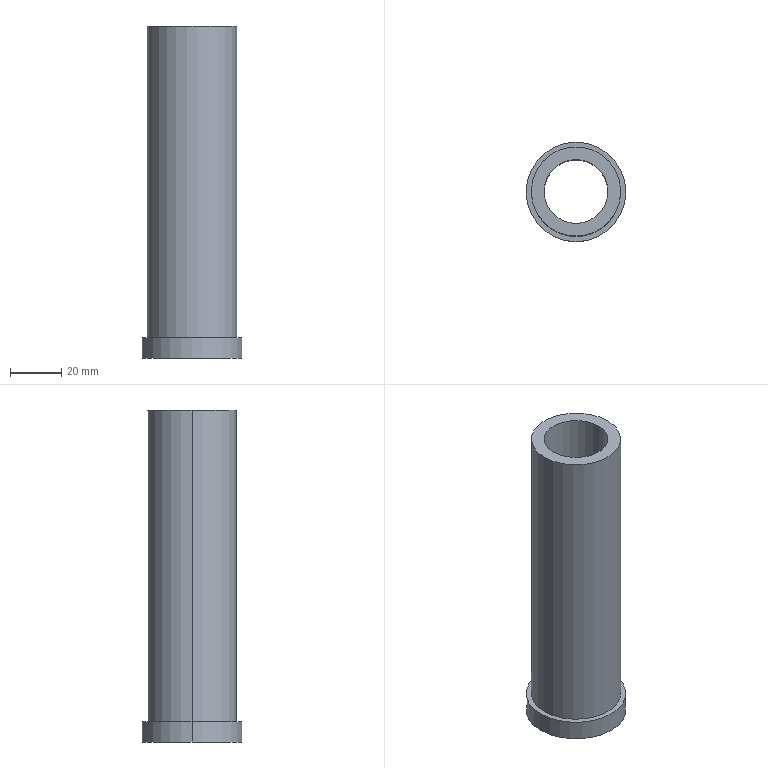Part | 1 solid | 9 faces | box 39 x 39 x 130 mm | volume 63121 mm3 | cylinder 6 | plane 3 | commonest cylinder face diameters 25 x2 35 x2 39 x2
STEP:
#1=CARTESIAN_POINT('',(17.5,0.,130.));
#2=VERTEX_POINT('',#1);
#3=CARTESIAN_POINT('',(-17.5,0.,130.));
#4=VERTEX_POINT('',#3);
#5=CARTESIAN_POINT('',(0.,0.,130.));
#6=DIRECTION('',(0.,0.,1.));
#7=DIRECTION('',(1.,0.,0.));
#8=AXIS2_PLACEMENT_3D('',#5,#6,#7);
#9=CIRCLE('',#8,17.5);
#10=EDGE_CURVE('',#2,#4,#9,.T.);
#11=ORIENTED_EDGE('',*,*,#10,.F.);
#12=CARTESIAN_POINT('',(17.5,0.,8.));
#13=VERTEX_POINT('',#12);
#14=CARTESIAN_POINT('',(17.5,0.,130.));
#15=DIRECTION('',(0.,0.,-1.));
#16=VECTOR('',#15,1000.);
#17=LINE('',#14,#16);
#18=EDGE_CURVE('',#2,#13,#17,.T.);
#19=ORIENTED_EDGE('',*,*,#18,.T.);
#20=CARTESIAN_POINT('',(-17.5,0.,8.));
#21=VERTEX_POINT('',#20);
#22=CARTESIAN_POINT('',(0.,0.,8.));
#23=DIRECTION('',(0.,0.,1.));
#24=DIRECTION('',(1.,0.,0.));
#25=AXIS2_PLACEMENT_3D('',#22,#23,#24);
#26=CIRCLE('',#25,17.5);
#27=EDGE_CURVE('',#13,#21,#26,.T.);
#28=ORIENTED_EDGE('',*,*,#27,.T.);
#29=CARTESIAN_POINT('',(-17.5,0.,130.));
#30=DIRECTION('',(0.,0.,-1.));
#31=VECTOR('',#30,1000.);
#32=LINE('',#29,#31);
#33=EDGE_CURVE('',#4,#21,#32,.T.);
#34=ORIENTED_EDGE('',*,*,#33,.F.);
#35=EDGE_LOOP('',(#11,#19,#28,#34));
#36=FACE_OUTER_BOUND('',#35,.T.);
#37=CARTESIAN_POINT('',(0.,0.,130.));
#38=DIRECTION('',(0.,0.,-1.));
#39=DIRECTION('',(-1.,0.,0.));
#40=AXIS2_PLACEMENT_3D('',#37,#38,#39);
#41=CYLINDRICAL_SURFACE('',#40,17.5);
#42=ADVANCED_FACE('',(#36),#41,.T.);
#43=CARTESIAN_POINT('',(-12.5,0.,130.));
#44=VERTEX_POINT('',#43);
#45=CARTESIAN_POINT('',(12.5,0.,130.));
#46=VERTEX_POINT('',#45);
#47=CARTESIAN_POINT('',(0.,0.,130.));
#48=DIRECTION('',(0.,0.,1.));
#49=DIRECTION('',(1.,0.,0.));
#50=AXIS2_PLACEMENT_3D('',#47,#48,#49);
#51=CIRCLE('',#50,12.5);
#52=EDGE_CURVE('',#44,#46,#51,.T.);
#53=ORIENTED_EDGE('',*,*,#52,.T.);
#54=CARTESIAN_POINT('',(12.5,0.,0.));
#55=VERTEX_POINT('',#54);
#56=CARTESIAN_POINT('',(12.5,0.,130.));
#57=DIRECTION('',(0.,0.,-1.));
#58=VECTOR('',#57,1000.);
#59=LINE('',#56,#58);
#60=EDGE_CURVE('',#46,#55,#59,.T.);
#61=ORIENTED_EDGE('',*,*,#60,.T.);
#62=CARTESIAN_POINT('',(-12.5,0.,0.));
#63=VERTEX_POINT('',#62);
#64=CARTESIAN_POINT('',(0.,0.,0.));
#65=DIRECTION('',(0.,0.,1.));
#66=DIRECTION('',(1.,0.,0.));
#67=AXIS2_PLACEMENT_3D('',#64,#65,#66);
#68=CIRCLE('',#67,12.5);
#69=EDGE_CURVE('',#63,#55,#68,.T.);
#70=ORIENTED_EDGE('',*,*,#69,.F.);
#71=CARTESIAN_POINT('',(-12.5,0.,130.));
#72=DIRECTION('',(0.,0.,-1.));
#73=VECTOR('',#72,1000.);
#74=LINE('',#71,#73);
#75=EDGE_CURVE('',#44,#63,#74,.T.);
#76=ORIENTED_EDGE('',*,*,#75,.F.);
#77=EDGE_LOOP('',(#53,#61,#70,#76));
#78=FACE_OUTER_BOUND('',#77,.T.);
#79=CARTESIAN_POINT('',(0.,0.,130.));
#80=DIRECTION('',(0.,0.,-1.));
#81=DIRECTION('',(-1.,0.,0.));
#82=AXIS2_PLACEMENT_3D('',#79,#80,#81);
#83=CYLINDRICAL_SURFACE('',#82,12.5);
#84=ADVANCED_FACE('',(#78),#83,.F.);
#85=CARTESIAN_POINT('',(19.5,0.,8.));
#86=VERTEX_POINT('',#85);
#87=CARTESIAN_POINT('',(-19.5,0.,8.));
#88=VERTEX_POINT('',#87);
#89=CARTESIAN_POINT('',(0.,0.,8.));
#90=DIRECTION('',(0.,0.,1.));
#91=DIRECTION('',(1.,0.,0.));
#92=AXIS2_PLACEMENT_3D('',#89,#90,#91);
#93=CIRCLE('',#92,19.5);
#94=EDGE_CURVE('',#86,#88,#93,.T.);
#95=ORIENTED_EDGE('',*,*,#94,.F.);
#96=CARTESIAN_POINT('',(19.5,0.,0.));
#97=VERTEX_POINT('',#96);
#98=CARTESIAN_POINT('',(19.5,0.,8.));
#99=DIRECTION('',(0.,0.,-1.));
#100=VECTOR('',#99,1000.);
#101=LINE('',#98,#100);
#102=EDGE_CURVE('',#86,#97,#101,.T.);
#103=ORIENTED_EDGE('',*,*,#102,.T.);
#104=CARTESIAN_POINT('',(-19.5,0.,0.));
#105=VERTEX_POINT('',#104);
#106=CARTESIAN_POINT('',(0.,0.,0.));
#107=DIRECTION('',(0.,0.,1.));
#108=DIRECTION('',(1.,0.,0.));
#109=AXIS2_PLACEMENT_3D('',#106,#107,#108);
#110=CIRCLE('',#109,19.5);
#111=EDGE_CURVE('',#97,#105,#110,.T.);
#112=ORIENTED_EDGE('',*,*,#111,.T.);
#113=CARTESIAN_POINT('',(-19.5,0.,8.));
#114=DIRECTION('',(0.,0.,-1.));
#115=VECTOR('',#114,1000.);
#116=LINE('',#113,#115);
#117=EDGE_CURVE('',#88,#105,#116,.T.);
#118=ORIENTED_EDGE('',*,*,#117,.F.);
#119=EDGE_LOOP('',(#95,#103,#112,#118));
#120=FACE_OUTER_BOUND('',#119,.T.);
#121=CARTESIAN_POINT('',(0.,0.,8.));
#122=DIRECTION('',(0.,0.,-1.));
#123=DIRECTION('',(-1.,0.,0.));
#124=AXIS2_PLACEMENT_3D('',#121,#122,#123);
#125=CYLINDRICAL_SURFACE('',#124,19.5);
#126=ADVANCED_FACE('',(#120),#125,.T.);
#127=ORIENTED_EDGE('',*,*,#102,.F.);
#128=CARTESIAN_POINT('',(0.,0.,8.));
#129=DIRECTION('',(0.,0.,1.));
#130=DIRECTION('',(1.,0.,0.));
#131=AXIS2_PLACEMENT_3D('',#128,#129,#130);
#132=CIRCLE('',#131,19.5);
#133=EDGE_CURVE('',#88,#86,#132,.T.);
#134=ORIENTED_EDGE('',*,*,#133,.F.);
#135=ORIENTED_EDGE('',*,*,#117,.T.);
#136=CARTESIAN_POINT('',(0.,0.,0.));
#137=DIRECTION('',(0.,0.,1.));
#138=DIRECTION('',(1.,0.,0.));
#139=AXIS2_PLACEMENT_3D('',#136,#137,#138);
#140=CIRCLE('',#139,19.5);
#141=EDGE_CURVE('',#105,#97,#140,.T.);
#142=ORIENTED_EDGE('',*,*,#141,.T.);
#143=EDGE_LOOP('',(#127,#134,#135,#142));
#144=FACE_OUTER_BOUND('',#143,.T.);
#145=CARTESIAN_POINT('',(0.,0.,8.));
#146=DIRECTION('',(0.,0.,-1.));
#147=DIRECTION('',(-1.,0.,0.));
#148=AXIS2_PLACEMENT_3D('',#145,#146,#147);
#149=CYLINDRICAL_SURFACE('',#148,19.5);
#150=ADVANCED_FACE('',(#144),#149,.T.);
#151=CARTESIAN_POINT('',(0.,0.,8.));
#152=DIRECTION('',(0.,0.,1.));
#153=DIRECTION('',(1.,0.,0.));
#154=AXIS2_PLACEMENT_3D('',#151,#152,#153);
#155=CIRCLE('',#154,17.5);
#156=EDGE_CURVE('',#21,#13,#155,.T.);
#157=ORIENTED_EDGE('',*,*,#156,.F.);
#158=ORIENTED_EDGE('',*,*,#27,.F.);
#159=EDGE_LOOP('',(#157,#158));
#160=FACE_BOUND('',#159,.T.);
#161=ORIENTED_EDGE('',*,*,#133,.T.);
#162=ORIENTED_EDGE('',*,*,#94,.T.);
#163=EDGE_LOOP('',(#161,#162));
#164=FACE_OUTER_BOUND('',#163,.T.);
#165=CARTESIAN_POINT('',(0.,0.,8.));
#166=DIRECTION('',(0.,0.,1.));
#167=DIRECTION('',(1.,0.,0.));
#168=AXIS2_PLACEMENT_3D('',#165,#166,#167);
#169=PLANE('',#168);
#170=ADVANCED_FACE('',(#160,#164),#169,.T.);
#171=ORIENTED_EDGE('',*,*,#141,.F.);
#172=ORIENTED_EDGE('',*,*,#111,.F.);
#173=EDGE_LOOP('',(#171,#172));
#174=FACE_OUTER_BOUND('',#173,.T.);
#175=ORIENTED_EDGE('',*,*,#69,.T.);
#176=CARTESIAN_POINT('',(0.,0.,0.));
#177=DIRECTION('',(0.,0.,1.));
#178=DIRECTION('',(1.,0.,0.));
#179=AXIS2_PLACEMENT_3D('',#176,#177,#178);
#180=CIRCLE('',#179,12.5);
#181=EDGE_CURVE('',#55,#63,#180,.T.);
#182=ORIENTED_EDGE('',*,*,#181,.T.);
#183=EDGE_LOOP('',(#175,#182));
#184=FACE_BOUND('',#183,.T.);
#185=CARTESIAN_POINT('',(0.,0.,0.));
#186=DIRECTION('',(0.,0.,1.));
#187=DIRECTION('',(1.,0.,0.));
#188=AXIS2_PLACEMENT_3D('',#185,#186,#187);
#189=PLANE('',#188);
#190=ADVANCED_FACE('',(#174,#184),#189,.F.);
#191=ORIENTED_EDGE('',*,*,#60,.F.);
#192=CARTESIAN_POINT('',(0.,0.,130.));
#193=DIRECTION('',(0.,0.,1.));
#194=DIRECTION('',(1.,0.,0.));
#195=AXIS2_PLACEMENT_3D('',#192,#193,#194);
#196=CIRCLE('',#195,12.5);
#197=EDGE_CURVE('',#46,#44,#196,.T.);
#198=ORIENTED_EDGE('',*,*,#197,.T.);
#199=ORIENTED_EDGE('',*,*,#75,.T.);
#200=ORIENTED_EDGE('',*,*,#181,.F.);
#201=EDGE_LOOP('',(#191,#198,#199,#200));
#202=FACE_OUTER_BOUND('',#201,.T.);
#203=CARTESIAN_POINT('',(0.,0.,130.));
#204=DIRECTION('',(0.,0.,-1.));
#205=DIRECTION('',(-1.,0.,0.));
#206=AXIS2_PLACEMENT_3D('',#203,#204,#205);
#207=CYLINDRICAL_SURFACE('',#206,12.5);
#208=ADVANCED_FACE('',(#202),#207,.F.);
#209=ORIENTED_EDGE('',*,*,#18,.F.);
#210=CARTESIAN_POINT('',(0.,0.,130.));
#211=DIRECTION('',(0.,0.,1.));
#212=DIRECTION('',(1.,0.,0.));
#213=AXIS2_PLACEMENT_3D('',#210,#211,#212);
#214=CIRCLE('',#213,17.5);
#215=EDGE_CURVE('',#4,#2,#214,.T.);
#216=ORIENTED_EDGE('',*,*,#215,.F.);
#217=ORIENTED_EDGE('',*,*,#33,.T.);
#218=ORIENTED_EDGE('',*,*,#156,.T.);
#219=EDGE_LOOP('',(#209,#216,#217,#218));
#220=FACE_OUTER_BOUND('',#219,.T.);
#221=CARTESIAN_POINT('',(0.,0.,130.));
#222=DIRECTION('',(0.,0.,-1.));
#223=DIRECTION('',(-1.,0.,0.));
#224=AXIS2_PLACEMENT_3D('',#221,#222,#223);
#225=CYLINDRICAL_SURFACE('',#224,17.5);
#226=ADVANCED_FACE('',(#220),#225,.T.);
#227=ORIENTED_EDGE('',*,*,#52,.F.);
#228=ORIENTED_EDGE('',*,*,#197,.F.);
#229=EDGE_LOOP('',(#227,#228));
#230=FACE_BOUND('',#229,.T.);
#231=ORIENTED_EDGE('',*,*,#215,.T.);
#232=ORIENTED_EDGE('',*,*,#10,.T.);
#233=EDGE_LOOP('',(#231,#232));
#234=FACE_OUTER_BOUND('',#233,.T.);
#235=CARTESIAN_POINT('',(0.,0.,130.));
#236=DIRECTION('',(0.,0.,1.));
#237=DIRECTION('',(1.,0.,0.));
#238=AXIS2_PLACEMENT_3D('',#235,#236,#237);
#239=PLANE('',#238);
#240=ADVANCED_FACE('',(#230,#234),#239,.T.);
#241=CLOSED_SHELL('',(#42,#84,#126,#150,#170,#190,#208,#226,#240));
#242=MANIFOLD_SOLID_BREP('',#241);
#243=CARTESIAN_POINT('',(0.,0.,0.));
#244=DIRECTION('',(0.,0.,1.));
#245=DIRECTION('',(1.,0.,0.));
#246=AXIS2_PLACEMENT_3D('',#243,#244,#245);
#247=(LENGTH_UNIT()NAMED_UNIT(*)SI_UNIT(.MILLI.,.METRE.));
#248=UNCERTAINTY_MEASURE_WITH_UNIT(LENGTH_MEASURE(0.00001),#247,'','');
#249=(NAMED_UNIT(*)PLANE_ANGLE_UNIT()SI_UNIT($,.RADIAN.));
#250=(NAMED_UNIT(*)SI_UNIT($,.STERADIAN.)SOLID_ANGLE_UNIT());
#251=(GEOMETRIC_REPRESENTATION_CONTEXT(3)GLOBAL_UNCERTAINTY_ASSIGNED_CONTEXT((#248))GLOBAL_UNIT_ASSIGNED_CONTEXT((#247,#249,#250))REPRESENTATION_CONTEXT('',''));
#252=ADVANCED_BREP_SHAPE_REPRESENTATION('',(#242,#246),#251);